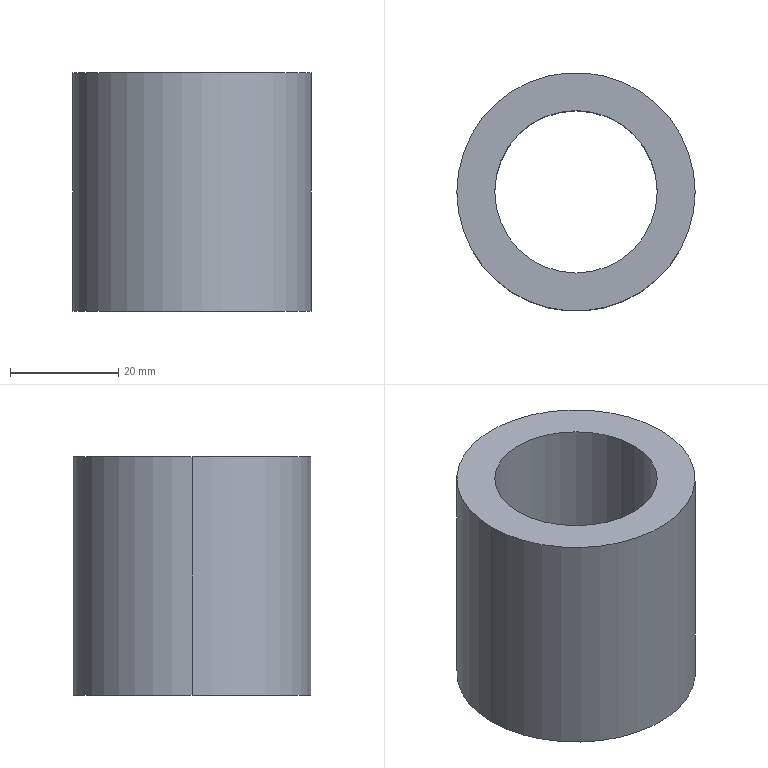Part | STEP file | Linear motion ball bearing | 1 solid | 6 faces | box 44 x 44 x 44 mm | volume 35802 mm3 | cylinder 4 | plane 2 | commonest cylinder face diameters 30 x2 44 x2
STEP:
#1=CARTESIAN_POINT('',(-22.,0.,44.));
#2=VERTEX_POINT('',#1);
#3=CARTESIAN_POINT('',(22.,0.,44.));
#4=VERTEX_POINT('',#3);
#5=CARTESIAN_POINT('',(0.,0.,44.));
#6=DIRECTION('',(0.,0.,-1.));
#7=DIRECTION('',(-1.,0.,0.));
#8=AXIS2_PLACEMENT_3D('',#5,#6,#7);
#9=CIRCLE('',#8,22.);
#10=EDGE_CURVE('',#2,#4,#9,.T.);
#11=ORIENTED_EDGE('',*,*,#10,.T.);
#12=CARTESIAN_POINT('',(22.,0.,0.));
#13=VERTEX_POINT('',#12);
#14=CARTESIAN_POINT('',(22.,0.,44.));
#15=DIRECTION('',(0.,0.,-1.));
#16=VECTOR('',#15,1000.);
#17=LINE('',#14,#16);
#18=EDGE_CURVE('',#4,#13,#17,.T.);
#19=ORIENTED_EDGE('',*,*,#18,.T.);
#20=CARTESIAN_POINT('',(-22.,0.,0.));
#21=VERTEX_POINT('',#20);
#22=CARTESIAN_POINT('',(0.,0.,0.));
#23=DIRECTION('',(0.,0.,1.));
#24=DIRECTION('',(-1.,0.,0.));
#25=AXIS2_PLACEMENT_3D('',#22,#23,#24);
#26=CIRCLE('',#25,22.);
#27=EDGE_CURVE('',#13,#21,#26,.T.);
#28=ORIENTED_EDGE('',*,*,#27,.T.);
#29=CARTESIAN_POINT('',(-22.,0.,44.));
#30=DIRECTION('',(0.,0.,-1.));
#31=VECTOR('',#30,1000.);
#32=LINE('',#29,#31);
#33=EDGE_CURVE('',#2,#21,#32,.T.);
#34=ORIENTED_EDGE('',*,*,#33,.F.);
#35=EDGE_LOOP('',(#11,#19,#28,#34));
#36=FACE_OUTER_BOUND('',#35,.T.);
#37=CARTESIAN_POINT('',(0.,0.,44.));
#38=DIRECTION('',(0.,0.,-1.));
#39=DIRECTION('',(-1.,0.,0.));
#40=AXIS2_PLACEMENT_3D('',#37,#38,#39);
#41=CYLINDRICAL_SURFACE('',#40,22.);
#42=ADVANCED_FACE('',(#36),#41,.T.);
#43=CARTESIAN_POINT('',(15.,0.,44.));
#44=VERTEX_POINT('',#43);
#45=CARTESIAN_POINT('',(-15.,0.,44.));
#46=VERTEX_POINT('',#45);
#47=CARTESIAN_POINT('',(0.,0.,44.));
#48=DIRECTION('',(0.,0.,-1.));
#49=DIRECTION('',(-1.,0.,0.));
#50=AXIS2_PLACEMENT_3D('',#47,#48,#49);
#51=CIRCLE('',#50,15.);
#52=EDGE_CURVE('',#44,#46,#51,.T.);
#53=ORIENTED_EDGE('',*,*,#52,.F.);
#54=CARTESIAN_POINT('',(15.,0.,0.));
#55=VERTEX_POINT('',#54);
#56=CARTESIAN_POINT('',(15.,0.,44.));
#57=DIRECTION('',(0.,0.,-1.));
#58=VECTOR('',#57,1000.);
#59=LINE('',#56,#58);
#60=EDGE_CURVE('',#44,#55,#59,.T.);
#61=ORIENTED_EDGE('',*,*,#60,.T.);
#62=CARTESIAN_POINT('',(-15.,0.,0.));
#63=VERTEX_POINT('',#62);
#64=CARTESIAN_POINT('',(0.,0.,0.));
#65=DIRECTION('',(0.,0.,-1.));
#66=DIRECTION('',(-1.,0.,0.));
#67=AXIS2_PLACEMENT_3D('',#64,#65,#66);
#68=CIRCLE('',#67,15.);
#69=EDGE_CURVE('',#55,#63,#68,.T.);
#70=ORIENTED_EDGE('',*,*,#69,.T.);
#71=CARTESIAN_POINT('',(-15.,0.,44.));
#72=DIRECTION('',(0.,0.,-1.));
#73=VECTOR('',#72,1000.);
#74=LINE('',#71,#73);
#75=EDGE_CURVE('',#46,#63,#74,.T.);
#76=ORIENTED_EDGE('',*,*,#75,.F.);
#77=EDGE_LOOP('',(#53,#61,#70,#76));
#78=FACE_OUTER_BOUND('',#77,.T.);
#79=CARTESIAN_POINT('',(0.,0.,44.));
#80=DIRECTION('',(0.,0.,-1.));
#81=DIRECTION('',(-1.,0.,0.));
#82=AXIS2_PLACEMENT_3D('',#79,#80,#81);
#83=CYLINDRICAL_SURFACE('',#82,15.);
#84=ADVANCED_FACE('',(#78),#83,.F.);
#85=ORIENTED_EDGE('',*,*,#18,.F.);
#86=CARTESIAN_POINT('',(0.,0.,44.));
#87=DIRECTION('',(0.,0.,-1.));
#88=DIRECTION('',(-1.,0.,0.));
#89=AXIS2_PLACEMENT_3D('',#86,#87,#88);
#90=CIRCLE('',#89,22.);
#91=EDGE_CURVE('',#4,#2,#90,.T.);
#92=ORIENTED_EDGE('',*,*,#91,.T.);
#93=ORIENTED_EDGE('',*,*,#33,.T.);
#94=CARTESIAN_POINT('',(0.,0.,0.));
#95=DIRECTION('',(0.,0.,1.));
#96=DIRECTION('',(-1.,0.,0.));
#97=AXIS2_PLACEMENT_3D('',#94,#95,#96);
#98=CIRCLE('',#97,22.);
#99=EDGE_CURVE('',#21,#13,#98,.T.);
#100=ORIENTED_EDGE('',*,*,#99,.T.);
#101=EDGE_LOOP('',(#85,#92,#93,#100));
#102=FACE_OUTER_BOUND('',#101,.T.);
#103=CARTESIAN_POINT('',(0.,0.,44.));
#104=DIRECTION('',(0.,0.,-1.));
#105=DIRECTION('',(-1.,0.,0.));
#106=AXIS2_PLACEMENT_3D('',#103,#104,#105);
#107=CYLINDRICAL_SURFACE('',#106,22.);
#108=ADVANCED_FACE('',(#102),#107,.T.);
#109=CARTESIAN_POINT('',(0.,0.,0.));
#110=DIRECTION('',(0.,0.,-1.));
#111=DIRECTION('',(-1.,0.,0.));
#112=AXIS2_PLACEMENT_3D('',#109,#110,#111);
#113=CIRCLE('',#112,15.);
#114=EDGE_CURVE('',#63,#55,#113,.T.);
#115=ORIENTED_EDGE('',*,*,#114,.F.);
#116=ORIENTED_EDGE('',*,*,#69,.F.);
#117=EDGE_LOOP('',(#115,#116));
#118=FACE_BOUND('',#117,.T.);
#119=ORIENTED_EDGE('',*,*,#99,.F.);
#120=ORIENTED_EDGE('',*,*,#27,.F.);
#121=EDGE_LOOP('',(#119,#120));
#122=FACE_OUTER_BOUND('',#121,.T.);
#123=CARTESIAN_POINT('',(0.,0.,0.));
#124=DIRECTION('',(0.,0.,1.));
#125=DIRECTION('',(1.,0.,0.));
#126=AXIS2_PLACEMENT_3D('',#123,#124,#125);
#127=PLANE('',#126);
#128=ADVANCED_FACE('',(#118,#122),#127,.F.);
#129=CARTESIAN_POINT('',(0.,0.,44.));
#130=DIRECTION('',(0.,0.,-1.));
#131=DIRECTION('',(-1.,0.,0.));
#132=AXIS2_PLACEMENT_3D('',#129,#130,#131);
#133=CIRCLE('',#132,15.);
#134=EDGE_CURVE('',#46,#44,#133,.T.);
#135=ORIENTED_EDGE('',*,*,#134,.T.);
#136=ORIENTED_EDGE('',*,*,#52,.T.);
#137=EDGE_LOOP('',(#135,#136));
#138=FACE_BOUND('',#137,.T.);
#139=ORIENTED_EDGE('',*,*,#10,.F.);
#140=ORIENTED_EDGE('',*,*,#91,.F.);
#141=EDGE_LOOP('',(#139,#140));
#142=FACE_OUTER_BOUND('',#141,.T.);
#143=CARTESIAN_POINT('',(0.,0.,44.));
#144=DIRECTION('',(0.,0.,1.));
#145=DIRECTION('',(1.,0.,0.));
#146=AXIS2_PLACEMENT_3D('',#143,#144,#145);
#147=PLANE('',#146);
#148=ADVANCED_FACE('',(#138,#142),#147,.T.);
#149=ORIENTED_EDGE('',*,*,#60,.F.);
#150=ORIENTED_EDGE('',*,*,#134,.F.);
#151=ORIENTED_EDGE('',*,*,#75,.T.);
#152=ORIENTED_EDGE('',*,*,#114,.T.);
#153=EDGE_LOOP('',(#149,#150,#151,#152));
#154=FACE_OUTER_BOUND('',#153,.T.);
#155=CARTESIAN_POINT('',(0.,0.,44.));
#156=DIRECTION('',(0.,0.,-1.));
#157=DIRECTION('',(-1.,0.,0.));
#158=AXIS2_PLACEMENT_3D('',#155,#156,#157);
#159=CYLINDRICAL_SURFACE('',#158,15.);
#160=ADVANCED_FACE('',(#154),#159,.F.);
#161=CLOSED_SHELL('',(#42,#84,#108,#128,#148,#160));
#162=MANIFOLD_SOLID_BREP('',#161);
#163=CARTESIAN_POINT('',(0.,0.,0.));
#164=DIRECTION('',(0.,0.,1.));
#165=DIRECTION('',(1.,0.,0.));
#166=AXIS2_PLACEMENT_3D('',#163,#164,#165);
#167=(LENGTH_UNIT()NAMED_UNIT(*)SI_UNIT(.MILLI.,.METRE.));
#168=UNCERTAINTY_MEASURE_WITH_UNIT(LENGTH_MEASURE(0.00001),#167,'','');
#169=(NAMED_UNIT(*)PLANE_ANGLE_UNIT()SI_UNIT($,.RADIAN.));
#170=(NAMED_UNIT(*)SI_UNIT($,.STERADIAN.)SOLID_ANGLE_UNIT());
#171=(GEOMETRIC_REPRESENTATION_CONTEXT(3)GLOBAL_UNCERTAINTY_ASSIGNED_CONTEXT((#168))GLOBAL_UNIT_ASSIGNED_CONTEXT((#167,#169,#170))REPRESENTATION_CONTEXT('',''));
#172=ADVANCED_BREP_SHAPE_REPRESENTATION('',(#162,#166),#171);